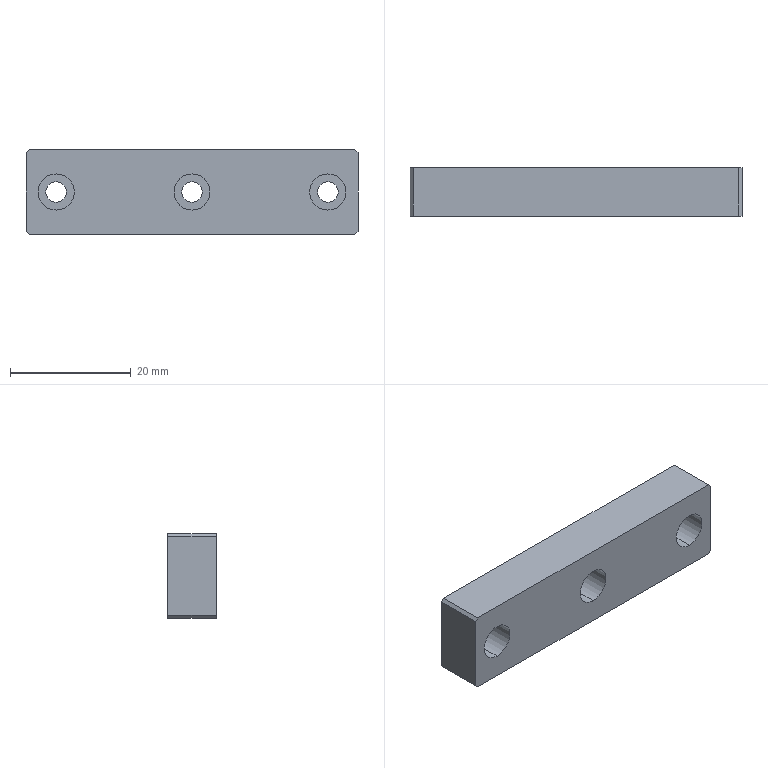Part | STEP file | 1 solid | 25 faces | box 55 x 8 x 14 mm | volume 5679 mm3 | plane 13 | cylinder 12 | commonest cylinder face diameters 3.4 x6 6 x6